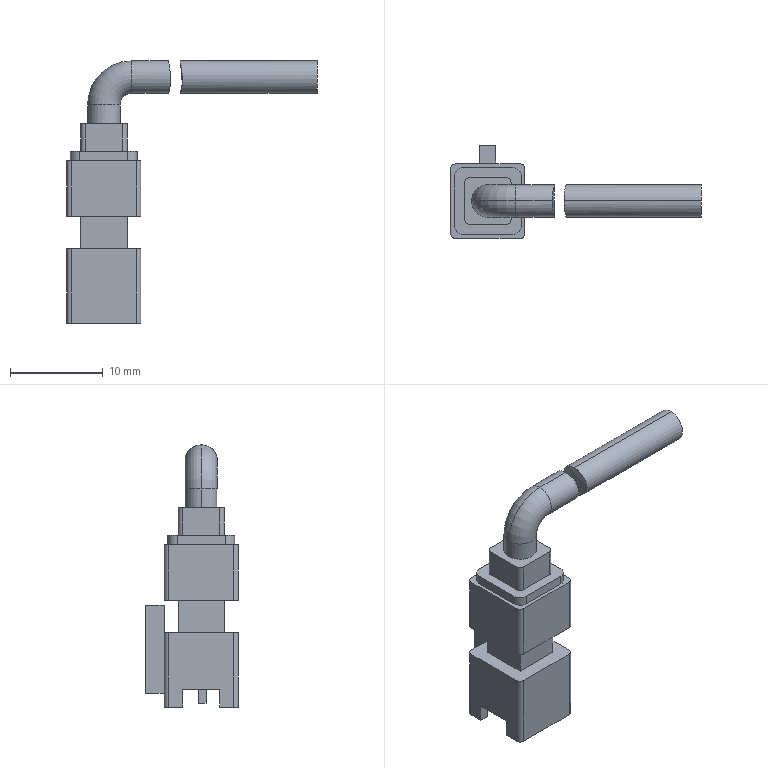Part | STEP file | ASND-0110-2-core outlet terminal | 2 solids | 85 faces | box 27 x 10 x 28.25 mm | volume 1155 mm3 | plane 59 | cylinder 22 | spline 2 | torus 2 | commonest cylinder face diameters 1 x12 3.5 x6 2 x4